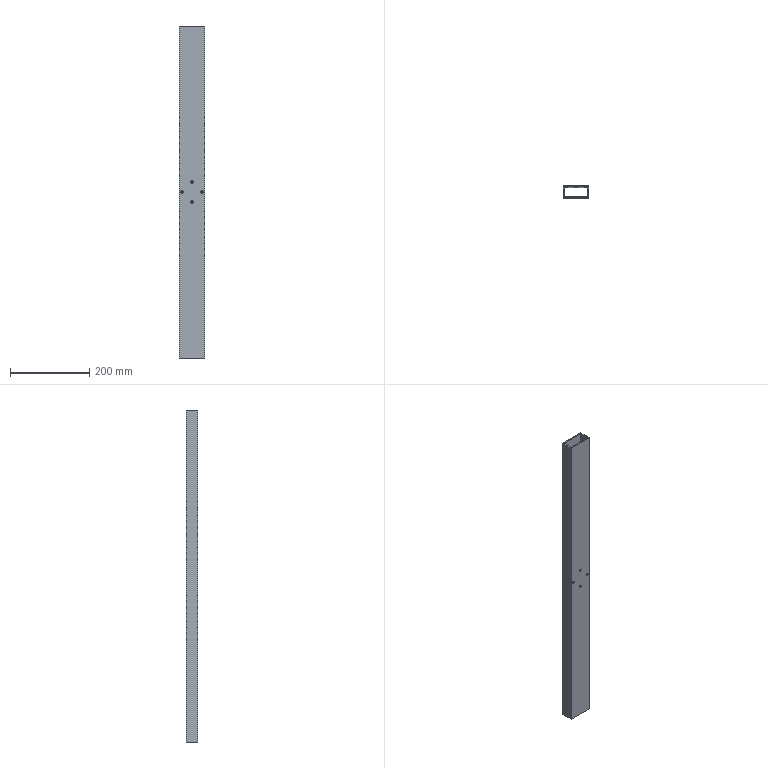Part | SolidWorks | features ICE 2, Extrusion 1 | 1 solid | 26 faces | box 65 x 30 x 840 mm | volume 447881 mm3 | cylinder 16 | plane 10 | commonest cylinder face diameters 6 x16
STEP:
#1=CARTESIAN_POINT('',(-8.041,12.808,398.));
#2=VERTEX_POINT('',#1);
#3=CARTESIAN_POINT('',(-8.041,12.808,392.));
#4=VERTEX_POINT('',#3);
#5=CARTESIAN_POINT('',(-8.041,12.808,395.));
#6=DIRECTION('',(0.,-1.,0.));
#7=DIRECTION('',(1.,0.,0.));
#8=AXIS2_PLACEMENT_3D('',#5,#6,#7);
#9=CIRCLE('',#8,3.);
#10=EDGE_CURVE('',#2,#4,#9,.T.);
#11=ORIENTED_EDGE('',*,*,#10,.F.);
#12=CARTESIAN_POINT('',(-8.041,9.808,398.));
#13=VERTEX_POINT('',#12);
#14=CARTESIAN_POINT('',(-8.041,39.808,398.));
#15=DIRECTION('',(0.,-1.,0.));
#16=VECTOR('',#15,1000.);
#17=LINE('',#14,#16);
#18=EDGE_CURVE('',#2,#13,#17,.T.);
#19=ORIENTED_EDGE('',*,*,#18,.T.);
#20=CARTESIAN_POINT('',(-8.041,9.808,392.));
#21=VERTEX_POINT('',#20);
#22=CARTESIAN_POINT('',(-8.041,9.808,395.));
#23=DIRECTION('',(0.,-1.,0.));
#24=DIRECTION('',(0.,0.,-1.));
#25=AXIS2_PLACEMENT_3D('',#22,#23,#24);
#26=CIRCLE('',#25,3.);
#27=EDGE_CURVE('',#13,#21,#26,.T.);
#28=ORIENTED_EDGE('',*,*,#27,.T.);
#29=CARTESIAN_POINT('',(-8.041,39.808,392.));
#30=DIRECTION('',(0.,-1.,0.));
#31=VECTOR('',#30,1000.);
#32=LINE('',#29,#31);
#33=EDGE_CURVE('',#4,#21,#32,.T.);
#34=ORIENTED_EDGE('',*,*,#33,.F.);
#35=EDGE_LOOP('',(#11,#19,#28,#34));
#36=FACE_OUTER_BOUND('',#35,.T.);
#37=CARTESIAN_POINT('',(-8.041,39.808,395.));
#38=DIRECTION('',(0.,-1.,0.));
#39=DIRECTION('',(0.,0.,-1.));
#40=AXIS2_PLACEMENT_3D('',#37,#38,#39);
#41=CYLINDRICAL_SURFACE('',#40,3.);
#42=ADVANCED_FACE('',(#36),#41,.F.);
#43=CARTESIAN_POINT('',(-33.041,12.808,423.));
#44=VERTEX_POINT('',#43);
#45=CARTESIAN_POINT('',(-33.041,12.808,417.));
#46=VERTEX_POINT('',#45);
#47=CARTESIAN_POINT('',(-33.041,12.808,420.));
#48=DIRECTION('',(0.,-1.,0.));
#49=DIRECTION('',(1.,0.,0.));
#50=AXIS2_PLACEMENT_3D('',#47,#48,#49);
#51=CIRCLE('',#50,3.);
#52=EDGE_CURVE('',#44,#46,#51,.T.);
#53=ORIENTED_EDGE('',*,*,#52,.F.);
#54=CARTESIAN_POINT('',(-33.041,9.808,423.));
#55=VERTEX_POINT('',#54);
#56=CARTESIAN_POINT('',(-33.041,39.808,423.));
#57=DIRECTION('',(0.,-1.,0.));
#58=VECTOR('',#57,1000.);
#59=LINE('',#56,#58);
#60=EDGE_CURVE('',#44,#55,#59,.T.);
#61=ORIENTED_EDGE('',*,*,#60,.T.);
#62=CARTESIAN_POINT('',(-33.041,9.808,417.));
#63=VERTEX_POINT('',#62);
#64=CARTESIAN_POINT('',(-33.041,9.808,420.));
#65=DIRECTION('',(0.,-1.,0.));
#66=DIRECTION('',(0.,0.,-1.));
#67=AXIS2_PLACEMENT_3D('',#64,#65,#66);
#68=CIRCLE('',#67,3.);
#69=EDGE_CURVE('',#55,#63,#68,.T.);
#70=ORIENTED_EDGE('',*,*,#69,.T.);
#71=CARTESIAN_POINT('',(-33.041,39.808,417.));
#72=DIRECTION('',(0.,-1.,0.));
#73=VECTOR('',#72,1000.);
#74=LINE('',#71,#73);
#75=EDGE_CURVE('',#46,#63,#74,.T.);
#76=ORIENTED_EDGE('',*,*,#75,.F.);
#77=EDGE_LOOP('',(#53,#61,#70,#76));
#78=FACE_OUTER_BOUND('',#77,.T.);
#79=CARTESIAN_POINT('',(-33.041,39.808,420.));
#80=DIRECTION('',(0.,-1.,0.));
#81=DIRECTION('',(0.,0.,-1.));
#82=AXIS2_PLACEMENT_3D('',#79,#80,#81);
#83=CYLINDRICAL_SURFACE('',#82,3.);
#84=ADVANCED_FACE('',(#78),#83,.F.);
#85=CARTESIAN_POINT('',(-8.041,12.808,448.));
#86=VERTEX_POINT('',#85);
#87=CARTESIAN_POINT('',(-8.041,12.808,442.));
#88=VERTEX_POINT('',#87);
#89=CARTESIAN_POINT('',(-8.041,12.808,445.));
#90=DIRECTION('',(0.,-1.,0.));
#91=DIRECTION('',(1.,0.,0.));
#92=AXIS2_PLACEMENT_3D('',#89,#90,#91);
#93=CIRCLE('',#92,3.);
#94=EDGE_CURVE('',#86,#88,#93,.T.);
#95=ORIENTED_EDGE('',*,*,#94,.F.);
#96=CARTESIAN_POINT('',(-8.041,9.808,448.));
#97=VERTEX_POINT('',#96);
#98=CARTESIAN_POINT('',(-8.041,39.808,448.));
#99=DIRECTION('',(0.,-1.,0.));
#100=VECTOR('',#99,1000.);
#101=LINE('',#98,#100);
#102=EDGE_CURVE('',#86,#97,#101,.T.);
#103=ORIENTED_EDGE('',*,*,#102,.T.);
#104=CARTESIAN_POINT('',(-8.041,9.808,442.));
#105=VERTEX_POINT('',#104);
#106=CARTESIAN_POINT('',(-8.041,9.808,445.));
#107=DIRECTION('',(0.,-1.,0.));
#108=DIRECTION('',(0.,0.,-1.));
#109=AXIS2_PLACEMENT_3D('',#106,#107,#108);
#110=CIRCLE('',#109,3.);
#111=EDGE_CURVE('',#97,#105,#110,.T.);
#112=ORIENTED_EDGE('',*,*,#111,.T.);
#113=CARTESIAN_POINT('',(-8.041,39.808,442.));
#114=DIRECTION('',(0.,-1.,0.));
#115=VECTOR('',#114,1000.);
#116=LINE('',#113,#115);
#117=EDGE_CURVE('',#88,#105,#116,.T.);
#118=ORIENTED_EDGE('',*,*,#117,.F.);
#119=EDGE_LOOP('',(#95,#103,#112,#118));
#120=FACE_OUTER_BOUND('',#119,.T.);
#121=CARTESIAN_POINT('',(-8.041,39.808,445.));
#122=DIRECTION('',(0.,-1.,0.));
#123=DIRECTION('',(0.,0.,-1.));
#124=AXIS2_PLACEMENT_3D('',#121,#122,#123);
#125=CYLINDRICAL_SURFACE('',#124,3.);
#126=ADVANCED_FACE('',(#120),#125,.F.);
#127=CARTESIAN_POINT('',(16.959,12.808,423.));
#128=VERTEX_POINT('',#127);
#129=CARTESIAN_POINT('',(16.959,12.808,417.));
#130=VERTEX_POINT('',#129);
#131=CARTESIAN_POINT('',(16.959,12.808,420.));
#132=DIRECTION('',(0.,-1.,0.));
#133=DIRECTION('',(1.,0.,0.));
#134=AXIS2_PLACEMENT_3D('',#131,#132,#133);
#135=CIRCLE('',#134,3.);
#136=EDGE_CURVE('',#128,#130,#135,.T.);
#137=ORIENTED_EDGE('',*,*,#136,.F.);
#138=CARTESIAN_POINT('',(16.959,9.808,423.));
#139=VERTEX_POINT('',#138);
#140=CARTESIAN_POINT('',(16.959,39.808,423.));
#141=DIRECTION('',(0.,-1.,0.));
#142=VECTOR('',#141,1000.);
#143=LINE('',#140,#142);
#144=EDGE_CURVE('',#128,#139,#143,.T.);
#145=ORIENTED_EDGE('',*,*,#144,.T.);
#146=CARTESIAN_POINT('',(16.959,9.808,417.));
#147=VERTEX_POINT('',#146);
#148=CARTESIAN_POINT('',(16.959,9.808,420.));
#149=DIRECTION('',(0.,-1.,0.));
#150=DIRECTION('',(0.,0.,-1.));
#151=AXIS2_PLACEMENT_3D('',#148,#149,#150);
#152=CIRCLE('',#151,3.);
#153=EDGE_CURVE('',#139,#147,#152,.T.);
#154=ORIENTED_EDGE('',*,*,#153,.T.);
#155=CARTESIAN_POINT('',(16.959,39.808,417.));
#156=DIRECTION('',(0.,-1.,0.));
#157=VECTOR('',#156,1000.);
#158=LINE('',#155,#157);
#159=EDGE_CURVE('',#130,#147,#158,.T.);
#160=ORIENTED_EDGE('',*,*,#159,.F.);
#161=EDGE_LOOP('',(#137,#145,#154,#160));
#162=FACE_OUTER_BOUND('',#161,.T.);
#163=CARTESIAN_POINT('',(16.959,39.808,420.));
#164=DIRECTION('',(0.,-1.,0.));
#165=DIRECTION('',(0.,0.,-1.));
#166=AXIS2_PLACEMENT_3D('',#163,#164,#165);
#167=CYLINDRICAL_SURFACE('',#166,3.);
#168=ADVANCED_FACE('',(#162),#167,.F.);
#169=CARTESIAN_POINT('',(-8.041,39.808,398.));
#170=VERTEX_POINT('',#169);
#171=CARTESIAN_POINT('',(-8.041,39.808,392.));
#172=VERTEX_POINT('',#171);
#173=CARTESIAN_POINT('',(-8.041,39.808,395.));
#174=DIRECTION('',(0.,-1.,0.));
#175=DIRECTION('',(0.,0.,-1.));
#176=AXIS2_PLACEMENT_3D('',#173,#174,#175);
#177=CIRCLE('',#176,3.);
#178=EDGE_CURVE('',#170,#172,#177,.T.);
#179=ORIENTED_EDGE('',*,*,#178,.F.);
#180=CARTESIAN_POINT('',(-8.041,36.808,398.));
#181=VERTEX_POINT('',#180);
#182=CARTESIAN_POINT('',(-8.041,39.808,398.));
#183=DIRECTION('',(0.,-1.,0.));
#184=VECTOR('',#183,1000.);
#185=LINE('',#182,#184);
#186=EDGE_CURVE('',#170,#181,#185,.T.);
#187=ORIENTED_EDGE('',*,*,#186,.T.);
#188=CARTESIAN_POINT('',(-8.041,36.808,392.));
#189=VERTEX_POINT('',#188);
#190=CARTESIAN_POINT('',(-8.041,36.808,395.));
#191=DIRECTION('',(0.,1.,0.));
#192=DIRECTION('',(-1.,0.,0.));
#193=AXIS2_PLACEMENT_3D('',#190,#191,#192);
#194=CIRCLE('',#193,3.);
#195=EDGE_CURVE('',#189,#181,#194,.T.);
#196=ORIENTED_EDGE('',*,*,#195,.F.);
#197=CARTESIAN_POINT('',(-8.041,39.808,392.));
#198=DIRECTION('',(0.,-1.,0.));
#199=VECTOR('',#198,1000.);
#200=LINE('',#197,#199);
#201=EDGE_CURVE('',#172,#189,#200,.T.);
#202=ORIENTED_EDGE('',*,*,#201,.F.);
#203=EDGE_LOOP('',(#179,#187,#196,#202));
#204=FACE_OUTER_BOUND('',#203,.T.);
#205=CARTESIAN_POINT('',(-8.041,39.808,395.));
#206=DIRECTION('',(0.,-1.,0.));
#207=DIRECTION('',(0.,0.,-1.));
#208=AXIS2_PLACEMENT_3D('',#205,#206,#207);
#209=CYLINDRICAL_SURFACE('',#208,3.);
#210=ADVANCED_FACE('',(#204),#209,.F.);
#211=CARTESIAN_POINT('',(-33.041,39.808,423.));
#212=VERTEX_POINT('',#211);
#213=CARTESIAN_POINT('',(-33.041,39.808,417.));
#214=VERTEX_POINT('',#213);
#215=CARTESIAN_POINT('',(-33.041,39.808,420.));
#216=DIRECTION('',(0.,-1.,0.));
#217=DIRECTION('',(0.,0.,-1.));
#218=AXIS2_PLACEMENT_3D('',#215,#216,#217);
#219=CIRCLE('',#218,3.);
#220=EDGE_CURVE('',#212,#214,#219,.T.);
#221=ORIENTED_EDGE('',*,*,#220,.F.);
#222=CARTESIAN_POINT('',(-33.041,36.808,423.));
#223=VERTEX_POINT('',#222);
#224=CARTESIAN_POINT('',(-33.041,39.808,423.));
#225=DIRECTION('',(0.,-1.,0.));
#226=VECTOR('',#225,1000.);
#227=LINE('',#224,#226);
#228=EDGE_CURVE('',#212,#223,#227,.T.);
#229=ORIENTED_EDGE('',*,*,#228,.T.);
#230=CARTESIAN_POINT('',(-33.041,36.808,417.));
#231=VERTEX_POINT('',#230);
#232=CARTESIAN_POINT('',(-33.041,36.808,420.));
#233=DIRECTION('',(0.,1.,0.));
#234=DIRECTION('',(-1.,0.,0.));
#235=AXIS2_PLACEMENT_3D('',#232,#233,#234);
#236=CIRCLE('',#235,3.);
#237=EDGE_CURVE('',#231,#223,#236,.T.);
#238=ORIENTED_EDGE('',*,*,#237,.F.);
#239=CARTESIAN_POINT('',(-33.041,39.808,417.));
#240=DIRECTION('',(0.,-1.,0.));
#241=VECTOR('',#240,1000.);
#242=LINE('',#239,#241);
#243=EDGE_CURVE('',#214,#231,#242,.T.);
#244=ORIENTED_EDGE('',*,*,#243,.F.);
#245=EDGE_LOOP('',(#221,#229,#238,#244));
#246=FACE_OUTER_BOUND('',#245,.T.);
#247=CARTESIAN_POINT('',(-33.041,39.808,420.));
#248=DIRECTION('',(0.,-1.,0.));
#249=DIRECTION('',(0.,0.,-1.));
#250=AXIS2_PLACEMENT_3D('',#247,#248,#249);
#251=CYLINDRICAL_SURFACE('',#250,3.);
#252=ADVANCED_FACE('',(#246),#251,.F.);
#253=CARTESIAN_POINT('',(-8.041,39.808,448.));
#254=VERTEX_POINT('',#253);
#255=CARTESIAN_POINT('',(-8.041,39.808,442.));
#256=VERTEX_POINT('',#255);
#257=CARTESIAN_POINT('',(-8.041,39.808,445.));
#258=DIRECTION('',(0.,-1.,0.));
#259=DIRECTION('',(0.,0.,-1.));
#260=AXIS2_PLACEMENT_3D('',#257,#258,#259);
#261=CIRCLE('',#260,3.);
#262=EDGE_CURVE('',#254,#256,#261,.T.);
#263=ORIENTED_EDGE('',*,*,#262,.F.);
#264=CARTESIAN_POINT('',(-8.041,36.808,448.));
#265=VERTEX_POINT('',#264);
#266=CARTESIAN_POINT('',(-8.041,39.808,448.));
#267=DIRECTION('',(0.,-1.,0.));
#268=VECTOR('',#267,1000.);
#269=LINE('',#266,#268);
#270=EDGE_CURVE('',#254,#265,#269,.T.);
#271=ORIENTED_EDGE('',*,*,#270,.T.);
#272=CARTESIAN_POINT('',(-8.041,36.808,442.));
#273=VERTEX_POINT('',#272);
#274=CARTESIAN_POINT('',(-8.041,36.808,445.));
#275=DIRECTION('',(0.,1.,0.));
#276=DIRECTION('',(-1.,0.,0.));
#277=AXIS2_PLACEMENT_3D('',#274,#275,#276);
#278=CIRCLE('',#277,3.);
#279=EDGE_CURVE('',#273,#265,#278,.T.);
#280=ORIENTED_EDGE('',*,*,#279,.F.);
#281=CARTESIAN_POINT('',(-8.041,39.808,442.));
#282=DIRECTION('',(0.,-1.,0.));
#283=VECTOR('',#282,1000.);
#284=LINE('',#281,#283);
#285=EDGE_CURVE('',#256,#273,#284,.T.);
#286=ORIENTED_EDGE('',*,*,#285,.F.);
#287=EDGE_LOOP('',(#263,#271,#280,#286));
#288=FACE_OUTER_BOUND('',#287,.T.);
#289=CARTESIAN_POINT('',(-8.041,39.808,445.));
#290=DIRECTION('',(0.,-1.,0.));
#291=DIRECTION('',(0.,0.,-1.));
#292=AXIS2_PLACEMENT_3D('',#289,#290,#291);
#293=CYLINDRICAL_SURFACE('',#292,3.);
#294=ADVANCED_FACE('',(#288),#293,.F.);
#295=CARTESIAN_POINT('',(16.959,39.808,423.));
#296=VERTEX_POINT('',#295);
#297=CARTESIAN_POINT('',(16.959,39.808,417.));
#298=VERTEX_POINT('',#297);
#299=CARTESIAN_POINT('',(16.959,39.808,420.));
#300=DIRECTION('',(0.,-1.,0.));
#301=DIRECTION('',(0.,0.,-1.));
#302=AXIS2_PLACEMENT_3D('',#299,#300,#301);
#303=CIRCLE('',#302,3.);
#304=EDGE_CURVE('',#296,#298,#303,.T.);
#305=ORIENTED_EDGE('',*,*,#304,.F.);
#306=CARTESIAN_POINT('',(16.959,36.808,423.));
#307=VERTEX_POINT('',#306);
#308=CARTESIAN_POINT('',(16.959,39.808,423.));
#309=DIRECTION('',(0.,-1.,0.));
#310=VECTOR('',#309,1000.);
#311=LINE('',#308,#310);
#312=EDGE_CURVE('',#296,#307,#311,.T.);
#313=ORIENTED_EDGE('',*,*,#312,.T.);
#314=CARTESIAN_POINT('',(16.959,36.808,417.));
#315=VERTEX_POINT('',#314);
#316=CARTESIAN_POINT('',(16.959,36.808,420.));
#317=DIRECTION('',(0.,1.,0.));
#318=DIRECTION('',(-1.,0.,0.));
#319=AXIS2_PLACEMENT_3D('',#316,#317,#318);
#320=CIRCLE('',#319,3.);
#321=EDGE_CURVE('',#315,#307,#320,.T.);
#322=ORIENTED_EDGE('',*,*,#321,.F.);
#323=CARTESIAN_POINT('',(16.959,39.808,417.));
#324=DIRECTION('',(0.,-1.,0.));
#325=VECTOR('',#324,1000.);
#326=LINE('',#323,#325);
#327=EDGE_CURVE('',#298,#315,#326,.T.);
#328=ORIENTED_EDGE('',*,*,#327,.F.);
#329=EDGE_LOOP('',(#305,#313,#322,#328));
#330=FACE_OUTER_BOUND('',#329,.T.);
#331=CARTESIAN_POINT('',(16.959,39.808,420.));
#332=DIRECTION('',(0.,-1.,0.));
#333=DIRECTION('',(0.,0.,-1.));
#334=AXIS2_PLACEMENT_3D('',#331,#332,#333);
#335=CYLINDRICAL_SURFACE('',#334,3.);
#336=ADVANCED_FACE('',(#330),#335,.F.);
#337=CARTESIAN_POINT('',(-40.541,39.808,0.));
#338=VERTEX_POINT('',#337);
#339=CARTESIAN_POINT('',(-40.541,9.808,0.));
#340=VERTEX_POINT('',#339);
#341=CARTESIAN_POINT('',(-40.541,9.808,0.));
#342=DIRECTION('',(0.,-1.,0.));
#343=VECTOR('',#342,1000.);
#344=LINE('',#341,#343);
#345=EDGE_CURVE('',#338,#340,#344,.T.);
#346=ORIENTED_EDGE('',*,*,#345,.T.);
#347=CARTESIAN_POINT('',(-40.541,9.808,840.));
#348=VERTEX_POINT('',#347);
#349=CARTESIAN_POINT('',(-40.541,9.808,840.));
#350=DIRECTION('',(0.,0.,-1.));
#351=VECTOR('',#350,1000.);
#352=LINE('',#349,#351);
#353=EDGE_CURVE('',#348,#340,#352,.T.);
#354=ORIENTED_EDGE('',*,*,#353,.F.);
#355=CARTESIAN_POINT('',(-40.541,39.808,840.));
#356=VERTEX_POINT('',#355);
#357=CARTESIAN_POINT('',(-40.541,9.808,840.));
#358=DIRECTION('',(0.,-1.,0.));
#359=VECTOR('',#358,1000.);
#360=LINE('',#357,#359);
#361=EDGE_CURVE('',#356,#348,#360,.T.);
#362=ORIENTED_EDGE('',*,*,#361,.F.);
#363=CARTESIAN_POINT('',(-40.541,39.808,840.));
#364=DIRECTION('',(0.,0.,-1.));
#365=VECTOR('',#364,1000.);
#366=LINE('',#363,#365);
#367=EDGE_CURVE('',#356,#338,#366,.T.);
#368=ORIENTED_EDGE('',*,*,#367,.T.);
#369=EDGE_LOOP('',(#346,#354,#362,#368));
#370=FACE_OUTER_BOUND('',#369,.T.);
#371=CARTESIAN_POINT('',(-40.541,9.808,840.));
#372=DIRECTION('',(1.,0.,0.));
#373=DIRECTION('',(0.,0.,-1.));
#374=AXIS2_PLACEMENT_3D('',#371,#372,#373);
#375=PLANE('',#374);
#376=ADVANCED_FACE('',(#370),#375,.F.);
#377=CARTESIAN_POINT('',(-8.041,9.808,395.));
#378=DIRECTION('',(0.,-1.,0.));
#379=DIRECTION('',(0.,0.,-1.));
#380=AXIS2_PLACEMENT_3D('',#377,#378,#379);
#381=CIRCLE('',#380,3.);
#382=EDGE_CURVE('',#21,#13,#381,.T.);
#383=ORIENTED_EDGE('',*,*,#382,.F.);
#384=ORIENTED_EDGE('',*,*,#27,.F.);
#385=EDGE_LOOP('',(#383,#384));
#386=FACE_BOUND('',#385,.T.);
#387=CARTESIAN_POINT('',(-33.041,9.808,420.));
#388=DIRECTION('',(0.,-1.,0.));
#389=DIRECTION('',(0.,0.,-1.));
#390=AXIS2_PLACEMENT_3D('',#387,#388,#389);
#391=CIRCLE('',#390,3.);
#392=EDGE_CURVE('',#63,#55,#391,.T.);
#393=ORIENTED_EDGE('',*,*,#392,.F.);
#394=ORIENTED_EDGE('',*,*,#69,.F.);
#395=EDGE_LOOP('',(#393,#394));
#396=FACE_BOUND('',#395,.T.);
#397=CARTESIAN_POINT('',(-8.041,9.808,445.));
#398=DIRECTION('',(0.,-1.,0.));
#399=DIRECTION('',(0.,0.,-1.));
#400=AXIS2_PLACEMENT_3D('',#397,#398,#399);
#401=CIRCLE('',#400,3.);
#402=EDGE_CURVE('',#105,#97,#401,.T.);
#403=ORIENTED_EDGE('',*,*,#402,.F.);
#404=ORIENTED_EDGE('',*,*,#111,.F.);
#405=EDGE_LOOP('',(#403,#404));
#406=FACE_BOUND('',#405,.T.);
#407=CARTESIAN_POINT('',(16.959,9.808,420.));
#408=DIRECTION('',(0.,-1.,0.));
#409=DIRECTION('',(0.,0.,-1.));
#410=AXIS2_PLACEMENT_3D('',#407,#408,#409);
#411=CIRCLE('',#410,3.);
#412=EDGE_CURVE('',#147,#139,#411,.T.);
#413=ORIENTED_EDGE('',*,*,#412,.F.);
#414=ORIENTED_EDGE('',*,*,#153,.F.);
#415=EDGE_LOOP('',(#413,#414));
#416=FACE_BOUND('',#415,.T.);
#417=CARTESIAN_POINT('',(24.459,9.808,0.));
#418=VERTEX_POINT('',#417);
#419=CARTESIAN_POINT('',(24.459,9.808,0.));
#420=DIRECTION('',(1.,0.,0.));
#421=VECTOR('',#420,1000.);
#422=LINE('',#419,#421);
#423=EDGE_CURVE('',#340,#418,#422,.T.);
#424=ORIENTED_EDGE('',*,*,#423,.T.);
#425=CARTESIAN_POINT('',(24.459,9.808,840.));
#426=VERTEX_POINT('',#425);
#427=CARTESIAN_POINT('',(24.459,9.808,840.));
#428=DIRECTION('',(0.,0.,-1.));
#429=VECTOR('',#428,1000.);
#430=LINE('',#427,#429);
#431=EDGE_CURVE('',#426,#418,#430,.T.);
#432=ORIENTED_EDGE('',*,*,#431,.F.);
#433=CARTESIAN_POINT('',(24.459,9.808,840.));
#434=DIRECTION('',(1.,0.,0.));
#435=VECTOR('',#434,1000.);
#436=LINE('',#433,#435);
#437=EDGE_CURVE('',#348,#426,#436,.T.);
#438=ORIENTED_EDGE('',*,*,#437,.F.);
#439=ORIENTED_EDGE('',*,*,#353,.T.);
#440=EDGE_LOOP('',(#424,#432,#438,#439));
#441=FACE_OUTER_BOUND('',#440,.T.);
#442=CARTESIAN_POINT('',(24.459,9.808,840.));
#443=DIRECTION('',(0.,1.,0.));
#444=DIRECTION('',(0.,0.,1.));
#445=AXIS2_PLACEMENT_3D('',#442,#443,#444);
#446=PLANE('',#445);
#447=ADVANCED_FACE('',(#386,#396,#406,#416,#441),#446,.F.);
#448=CARTESIAN_POINT('',(24.459,39.808,0.));
#449=VERTEX_POINT('',#448);
#450=CARTESIAN_POINT('',(24.459,39.808,0.));
#451=DIRECTION('',(0.,1.,0.));
#452=VECTOR('',#451,1000.);
#453=LINE('',#450,#452);
#454=EDGE_CURVE('',#418,#449,#453,.T.);
#455=ORIENTED_EDGE('',*,*,#454,.T.);
#456=CARTESIAN_POINT('',(24.459,39.808,840.));
#457=VERTEX_POINT('',#456);
#458=CARTESIAN_POINT('',(24.459,39.808,840.));
#459=DIRECTION('',(0.,0.,-1.));
#460=VECTOR('',#459,1000.);
#461=LINE('',#458,#460);
#462=EDGE_CURVE('',#457,#449,#461,.T.);
#463=ORIENTED_EDGE('',*,*,#462,.F.);
#464=CARTESIAN_POINT('',(24.459,39.808,840.));
#465=DIRECTION('',(0.,1.,0.));
#466=VECTOR('',#465,1000.);
#467=LINE('',#464,#466);
#468=EDGE_CURVE('',#426,#457,#467,.T.);
#469=ORIENTED_EDGE('',*,*,#468,.F.);
#470=ORIENTED_EDGE('',*,*,#431,.T.);
#471=EDGE_LOOP('',(#455,#463,#469,#470));
#472=FACE_OUTER_BOUND('',#471,.T.);
#473=CARTESIAN_POINT('',(24.459,39.808,840.));
#474=DIRECTION('',(-1.,0.,0.));
#475=DIRECTION('',(0.,0.,1.));
#476=AXIS2_PLACEMENT_3D('',#473,#474,#475);
#477=PLANE('',#476);
#478=ADVANCED_FACE('',(#472),#477,.F.);
#479=CARTESIAN_POINT('',(-8.041,39.808,395.));
#480=DIRECTION('',(0.,-1.,0.));
#481=DIRECTION('',(0.,0.,-1.));
#482=AXIS2_PLACEMENT_3D('',#479,#480,#481);
#483=CIRCLE('',#482,3.);
#484=EDGE_CURVE('',#172,#170,#483,.T.);
#485=ORIENTED_EDGE('',*,*,#484,.T.);
#486=ORIENTED_EDGE('',*,*,#178,.T.);
#487=EDGE_LOOP('',(#485,#486));
#488=FACE_BOUND('',#487,.T.);
#489=CARTESIAN_POINT('',(-33.041,39.808,420.));
#490=DIRECTION('',(0.,-1.,0.));
#491=DIRECTION('',(0.,0.,-1.));
#492=AXIS2_PLACEMENT_3D('',#489,#490,#491);
#493=CIRCLE('',#492,3.);
#494=EDGE_CURVE('',#214,#212,#493,.T.);
#495=ORIENTED_EDGE('',*,*,#494,.T.);
#496=ORIENTED_EDGE('',*,*,#220,.T.);
#497=EDGE_LOOP('',(#495,#496));
#498=FACE_BOUND('',#497,.T.);
#499=CARTESIAN_POINT('',(-8.041,39.808,445.));
#500=DIRECTION('',(0.,-1.,0.));
#501=DIRECTION('',(0.,0.,-1.));
#502=AXIS2_PLACEMENT_3D('',#499,#500,#501);
#503=CIRCLE('',#502,3.);
#504=EDGE_CURVE('',#256,#254,#503,.T.);
#505=ORIENTED_EDGE('',*,*,#504,.T.);
#506=ORIENTED_EDGE('',*,*,#262,.T.);
#507=EDGE_LOOP('',(#505,#506));
#508=FACE_BOUND('',#507,.T.);
#509=CARTESIAN_POINT('',(16.959,39.808,420.));
#510=DIRECTION('',(0.,-1.,0.));
#511=DIRECTION('',(0.,0.,-1.));
#512=AXIS2_PLACEMENT_3D('',#509,#510,#511);
#513=CIRCLE('',#512,3.);
#514=EDGE_CURVE('',#298,#296,#513,.T.);
#515=ORIENTED_EDGE('',*,*,#514,.T.);
#516=ORIENTED_EDGE('',*,*,#304,.T.);
#517=EDGE_LOOP('',(#515,#516));
#518=FACE_BOUND('',#517,.T.);
#519=CARTESIAN_POINT('',(-40.541,39.808,0.));
#520=DIRECTION('',(-1.,0.,0.));
#521=VECTOR('',#520,1000.);
#522=LINE('',#519,#521);
#523=EDGE_CURVE('',#449,#338,#522,.T.);
#524=ORIENTED_EDGE('',*,*,#523,.T.);
#525=ORIENTED_EDGE('',*,*,#367,.F.);
#526=CARTESIAN_POINT('',(-40.541,39.808,840.));
#527=DIRECTION('',(-1.,0.,0.));
#528=VECTOR('',#527,1000.);
#529=LINE('',#526,#528);
#530=EDGE_CURVE('',#457,#356,#529,.T.);
#531=ORIENTED_EDGE('',*,*,#530,.F.);
#532=ORIENTED_EDGE('',*,*,#462,.T.);
#533=EDGE_LOOP('',(#524,#525,#531,#532));
#534=FACE_OUTER_BOUND('',#533,.T.);
#535=CARTESIAN_POINT('',(-40.541,39.808,840.));
#536=DIRECTION('',(0.,-1.,0.));
#537=DIRECTION('',(0.,0.,-1.));
#538=AXIS2_PLACEMENT_3D('',#535,#536,#537);
#539=PLANE('',#538);
#540=ADVANCED_FACE('',(#488,#498,#508,#518,#534),#539,.F.);
#541=CARTESIAN_POINT('',(21.459,36.808,840.));
#542=VERTEX_POINT('',#541);
#543=CARTESIAN_POINT('',(-37.541,36.808,840.));
#544=VERTEX_POINT('',#543);
#545=CARTESIAN_POINT('',(-37.541,36.808,840.));
#546=DIRECTION('',(-1.,0.,0.));
#547=VECTOR('',#546,1000.);
#548=LINE('',#545,#547);
#549=EDGE_CURVE('',#542,#544,#548,.T.);
#550=ORIENTED_EDGE('',*,*,#549,.F.);
#551=CARTESIAN_POINT('',(21.459,12.808,840.));
#552=VERTEX_POINT('',#551);
#553=CARTESIAN_POINT('',(21.459,36.808,840.));
#554=DIRECTION('',(0.,1.,0.));
#555=VECTOR('',#554,1000.);
#556=LINE('',#553,#555);
#557=EDGE_CURVE('',#552,#542,#556,.T.);
#558=ORIENTED_EDGE('',*,*,#557,.F.);
#559=CARTESIAN_POINT('',(-37.541,12.808,840.));
#560=VERTEX_POINT('',#559);
#561=CARTESIAN_POINT('',(21.459,12.808,840.));
#562=DIRECTION('',(1.,0.,0.));
#563=VECTOR('',#562,1000.);
#564=LINE('',#561,#563);
#565=EDGE_CURVE('',#560,#552,#564,.T.);
#566=ORIENTED_EDGE('',*,*,#565,.F.);
#567=CARTESIAN_POINT('',(-37.541,12.808,840.));
#568=DIRECTION('',(0.,-1.,0.));
#569=VECTOR('',#568,1000.);
#570=LINE('',#567,#569);
#571=EDGE_CURVE('',#544,#560,#570,.T.);
#572=ORIENTED_EDGE('',*,*,#571,.F.);
#573=EDGE_LOOP('',(#550,#558,#566,#572));
#574=FACE_BOUND('',#573,.T.);
#575=ORIENTED_EDGE('',*,*,#361,.T.);
#576=ORIENTED_EDGE('',*,*,#437,.T.);
#577=ORIENTED_EDGE('',*,*,#468,.T.);
#578=ORIENTED_EDGE('',*,*,#530,.T.);
#579=EDGE_LOOP('',(#575,#576,#577,#578));
#580=FACE_OUTER_BOUND('',#579,.T.);
#581=CARTESIAN_POINT('',(0.,0.,840.));
#582=DIRECTION('',(0.,0.,-1.));
#583=DIRECTION('',(-1.,0.,0.));
#584=AXIS2_PLACEMENT_3D('',#581,#582,#583);
#585=PLANE('',#584);
#586=ADVANCED_FACE('',(#574,#580),#585,.F.);
#587=CARTESIAN_POINT('',(21.459,36.808,0.));
#588=VERTEX_POINT('',#587);
#589=CARTESIAN_POINT('',(21.459,12.808,0.));
#590=VERTEX_POINT('',#589);
#591=CARTESIAN_POINT('',(21.459,0.,0.));
#592=DIRECTION('',(0.,-1.,0.));
#593=VECTOR('',#592,1000.);
#594=LINE('',#591,#593);
#595=EDGE_CURVE('',#588,#590,#594,.T.);
#596=ORIENTED_EDGE('',*,*,#595,.F.);
#597=CARTESIAN_POINT('',(-37.541,36.808,0.));
#598=VERTEX_POINT('',#597);
#599=CARTESIAN_POINT('',(0.,36.808,0.));
#600=DIRECTION('',(1.,0.,0.));
#601=VECTOR('',#600,1000.);
#602=LINE('',#599,#601);
#603=EDGE_CURVE('',#598,#588,#602,.T.);
#604=ORIENTED_EDGE('',*,*,#603,.F.);
#605=CARTESIAN_POINT('',(-37.541,12.808,0.));
#606=VERTEX_POINT('',#605);
#607=CARTESIAN_POINT('',(-37.541,0.,0.));
#608=DIRECTION('',(0.,1.,0.));
#609=VECTOR('',#608,1000.);
#610=LINE('',#607,#609);
#611=EDGE_CURVE('',#606,#598,#610,.T.);
#612=ORIENTED_EDGE('',*,*,#611,.F.);
#613=CARTESIAN_POINT('',(0.,12.808,0.));
#614=DIRECTION('',(-1.,0.,0.));
#615=VECTOR('',#614,1000.);
#616=LINE('',#613,#615);
#617=EDGE_CURVE('',#590,#606,#616,.T.);
#618=ORIENTED_EDGE('',*,*,#617,.F.);
#619=EDGE_LOOP('',(#596,#604,#612,#618));
#620=FACE_BOUND('',#619,.T.);
#621=ORIENTED_EDGE('',*,*,#345,.F.);
#622=ORIENTED_EDGE('',*,*,#523,.F.);
#623=ORIENTED_EDGE('',*,*,#454,.F.);
#624=ORIENTED_EDGE('',*,*,#423,.F.);
#625=EDGE_LOOP('',(#621,#622,#623,#624));
#626=FACE_OUTER_BOUND('',#625,.T.);
#627=CARTESIAN_POINT('',(0.,0.,0.));
#628=DIRECTION('',(0.,0.,-1.));
#629=DIRECTION('',(-1.,0.,0.));
#630=AXIS2_PLACEMENT_3D('',#627,#628,#629);
#631=PLANE('',#630);
#632=ADVANCED_FACE('',(#620,#626),#631,.T.);
#633=ORIENTED_EDGE('',*,*,#595,.T.);
#634=CARTESIAN_POINT('',(21.459,12.808,-110.));
#635=DIRECTION('',(0.,0.,1.));
#636=VECTOR('',#635,1000.);
#637=LINE('',#634,#636);
#638=EDGE_CURVE('',#590,#552,#637,.T.);
#639=ORIENTED_EDGE('',*,*,#638,.T.);
#640=ORIENTED_EDGE('',*,*,#557,.T.);
#641=CARTESIAN_POINT('',(21.459,36.808,-110.));
#642=DIRECTION('',(0.,0.,1.));
#643=VECTOR('',#642,1000.);
#644=LINE('',#641,#643);
#645=EDGE_CURVE('',#588,#542,#644,.T.);
#646=ORIENTED_EDGE('',*,*,#645,.F.);
#647=EDGE_LOOP('',(#633,#639,#640,#646));
#648=FACE_OUTER_BOUND('',#647,.T.);
#649=CARTESIAN_POINT('',(21.459,36.808,-110.));
#650=DIRECTION('',(1.,0.,0.));
#651=DIRECTION('',(0.,1.,0.));
#652=AXIS2_PLACEMENT_3D('',#649,#650,#651);
#653=PLANE('',#652);
#654=ADVANCED_FACE('',(#648),#653,.F.);
#655=CARTESIAN_POINT('',(-8.041,12.808,395.));
#656=DIRECTION('',(0.,-1.,0.));
#657=DIRECTION('',(1.,0.,0.));
#658=AXIS2_PLACEMENT_3D('',#655,#656,#657);
#659=CIRCLE('',#658,3.);
#660=EDGE_CURVE('',#4,#2,#659,.T.);
#661=ORIENTED_EDGE('',*,*,#660,.T.);
#662=ORIENTED_EDGE('',*,*,#10,.T.);
#663=EDGE_LOOP('',(#661,#662));
#664=FACE_BOUND('',#663,.T.);
#665=CARTESIAN_POINT('',(-33.041,12.808,420.));
#666=DIRECTION('',(0.,-1.,0.));
#667=DIRECTION('',(1.,0.,0.));
#668=AXIS2_PLACEMENT_3D('',#665,#666,#667);
#669=CIRCLE('',#668,3.);
#670=EDGE_CURVE('',#46,#44,#669,.T.);
#671=ORIENTED_EDGE('',*,*,#670,.T.);
#672=ORIENTED_EDGE('',*,*,#52,.T.);
#673=EDGE_LOOP('',(#671,#672));
#674=FACE_BOUND('',#673,.T.);
#675=CARTESIAN_POINT('',(-8.041,12.808,445.));
#676=DIRECTION('',(0.,-1.,0.));
#677=DIRECTION('',(1.,0.,0.));
#678=AXIS2_PLACEMENT_3D('',#675,#676,#677);
#679=CIRCLE('',#678,3.);
#680=EDGE_CURVE('',#88,#86,#679,.T.);
#681=ORIENTED_EDGE('',*,*,#680,.T.);
#682=ORIENTED_EDGE('',*,*,#94,.T.);
#683=EDGE_LOOP('',(#681,#682));
#684=FACE_BOUND('',#683,.T.);
#685=CARTESIAN_POINT('',(16.959,12.808,420.));
#686=DIRECTION('',(0.,-1.,0.));
#687=DIRECTION('',(1.,0.,0.));
#688=AXIS2_PLACEMENT_3D('',#685,#686,#687);
#689=CIRCLE('',#688,3.);
#690=EDGE_CURVE('',#130,#128,#689,.T.);
#691=ORIENTED_EDGE('',*,*,#690,.T.);
#692=ORIENTED_EDGE('',*,*,#136,.T.);
#693=EDGE_LOOP('',(#691,#692));
#694=FACE_BOUND('',#693,.T.);
#695=ORIENTED_EDGE('',*,*,#617,.T.);
#696=CARTESIAN_POINT('',(-37.541,12.808,-110.));
#697=DIRECTION('',(0.,0.,1.));
#698=VECTOR('',#697,1000.);
#699=LINE('',#696,#698);
#700=EDGE_CURVE('',#606,#560,#699,.T.);
#701=ORIENTED_EDGE('',*,*,#700,.T.);
#702=ORIENTED_EDGE('',*,*,#565,.T.);
#703=ORIENTED_EDGE('',*,*,#638,.F.);
#704=EDGE_LOOP('',(#695,#701,#702,#703));
#705=FACE_OUTER_BOUND('',#704,.T.);
#706=CARTESIAN_POINT('',(21.459,12.808,-110.));
#707=DIRECTION('',(0.,-1.,0.));
#708=DIRECTION('',(1.,0.,0.));
#709=AXIS2_PLACEMENT_3D('',#706,#707,#708);
#710=PLANE('',#709);
#711=ADVANCED_FACE('',(#664,#674,#684,#694,#705),#710,.F.);
#712=ORIENTED_EDGE('',*,*,#611,.T.);
#713=CARTESIAN_POINT('',(-37.541,36.808,-110.));
#714=DIRECTION('',(0.,0.,1.));
#715=VECTOR('',#714,1000.);
#716=LINE('',#713,#715);
#717=EDGE_CURVE('',#598,#544,#716,.T.);
#718=ORIENTED_EDGE('',*,*,#717,.T.);
#719=ORIENTED_EDGE('',*,*,#571,.T.);
#720=ORIENTED_EDGE('',*,*,#700,.F.);
#721=EDGE_LOOP('',(#712,#718,#719,#720));
#722=FACE_OUTER_BOUND('',#721,.T.);
#723=CARTESIAN_POINT('',(-37.541,12.808,-110.));
#724=DIRECTION('',(-1.,0.,0.));
#725=DIRECTION('',(0.,0.,1.));
#726=AXIS2_PLACEMENT_3D('',#723,#724,#725);
#727=PLANE('',#726);
#728=ADVANCED_FACE('',(#722),#727,.F.);
#729=ORIENTED_EDGE('',*,*,#195,.T.);
#730=CARTESIAN_POINT('',(-8.041,36.808,395.));
#731=DIRECTION('',(0.,1.,0.));
#732=DIRECTION('',(-1.,0.,0.));
#733=AXIS2_PLACEMENT_3D('',#730,#731,#732);
#734=CIRCLE('',#733,3.);
#735=EDGE_CURVE('',#181,#189,#734,.T.);
#736=ORIENTED_EDGE('',*,*,#735,.T.);
#737=EDGE_LOOP('',(#729,#736));
#738=FACE_BOUND('',#737,.T.);
#739=ORIENTED_EDGE('',*,*,#237,.T.);
#740=CARTESIAN_POINT('',(-33.041,36.808,420.));
#741=DIRECTION('',(0.,1.,0.));
#742=DIRECTION('',(-1.,0.,0.));
#743=AXIS2_PLACEMENT_3D('',#740,#741,#742);
#744=CIRCLE('',#743,3.);
#745=EDGE_CURVE('',#223,#231,#744,.T.);
#746=ORIENTED_EDGE('',*,*,#745,.T.);
#747=EDGE_LOOP('',(#739,#746));
#748=FACE_BOUND('',#747,.T.);
#749=ORIENTED_EDGE('',*,*,#279,.T.);
#750=CARTESIAN_POINT('',(-8.041,36.808,445.));
#751=DIRECTION('',(0.,1.,0.));
#752=DIRECTION('',(-1.,0.,0.));
#753=AXIS2_PLACEMENT_3D('',#750,#751,#752);
#754=CIRCLE('',#753,3.);
#755=EDGE_CURVE('',#265,#273,#754,.T.);
#756=ORIENTED_EDGE('',*,*,#755,.T.);
#757=EDGE_LOOP('',(#749,#756));
#758=FACE_BOUND('',#757,.T.);
#759=ORIENTED_EDGE('',*,*,#321,.T.);
#760=CARTESIAN_POINT('',(16.959,36.808,420.));
#761=DIRECTION('',(0.,1.,0.));
#762=DIRECTION('',(-1.,0.,0.));
#763=AXIS2_PLACEMENT_3D('',#760,#761,#762);
#764=CIRCLE('',#763,3.);
#765=EDGE_CURVE('',#307,#315,#764,.T.);
#766=ORIENTED_EDGE('',*,*,#765,.T.);
#767=EDGE_LOOP('',(#759,#766));
#768=FACE_BOUND('',#767,.T.);
#769=ORIENTED_EDGE('',*,*,#603,.T.);
#770=ORIENTED_EDGE('',*,*,#645,.T.);
#771=ORIENTED_EDGE('',*,*,#549,.T.);
#772=ORIENTED_EDGE('',*,*,#717,.F.);
#773=EDGE_LOOP('',(#769,#770,#771,#772));
#774=FACE_OUTER_BOUND('',#773,.T.);
#775=CARTESIAN_POINT('',(-37.541,36.808,-110.));
#776=DIRECTION('',(0.,1.,0.));
#777=DIRECTION('',(-1.,0.,0.));
#778=AXIS2_PLACEMENT_3D('',#775,#776,#777);
#779=PLANE('',#778);
#780=ADVANCED_FACE('',(#738,#748,#758,#768,#774),#779,.F.);
#781=ORIENTED_EDGE('',*,*,#312,.F.);
#782=ORIENTED_EDGE('',*,*,#514,.F.);
#783=ORIENTED_EDGE('',*,*,#327,.T.);
#784=ORIENTED_EDGE('',*,*,#765,.F.);
#785=EDGE_LOOP('',(#781,#782,#783,#784));
#786=FACE_OUTER_BOUND('',#785,.T.);
#787=CARTESIAN_POINT('',(16.959,39.808,420.));
#788=DIRECTION('',(0.,-1.,0.));
#789=DIRECTION('',(0.,0.,-1.));
#790=AXIS2_PLACEMENT_3D('',#787,#788,#789);
#791=CYLINDRICAL_SURFACE('',#790,3.);
#792=ADVANCED_FACE('',(#786),#791,.F.);
#793=ORIENTED_EDGE('',*,*,#270,.F.);
#794=ORIENTED_EDGE('',*,*,#504,.F.);
#795=ORIENTED_EDGE('',*,*,#285,.T.);
#796=ORIENTED_EDGE('',*,*,#755,.F.);
#797=EDGE_LOOP('',(#793,#794,#795,#796));
#798=FACE_OUTER_BOUND('',#797,.T.);
#799=CARTESIAN_POINT('',(-8.041,39.808,445.));
#800=DIRECTION('',(0.,-1.,0.));
#801=DIRECTION('',(0.,0.,-1.));
#802=AXIS2_PLACEMENT_3D('',#799,#800,#801);
#803=CYLINDRICAL_SURFACE('',#802,3.);
#804=ADVANCED_FACE('',(#798),#803,.F.);
#805=ORIENTED_EDGE('',*,*,#228,.F.);
#806=ORIENTED_EDGE('',*,*,#494,.F.);
#807=ORIENTED_EDGE('',*,*,#243,.T.);
#808=ORIENTED_EDGE('',*,*,#745,.F.);
#809=EDGE_LOOP('',(#805,#806,#807,#808));
#810=FACE_OUTER_BOUND('',#809,.T.);
#811=CARTESIAN_POINT('',(-33.041,39.808,420.));
#812=DIRECTION('',(0.,-1.,0.));
#813=DIRECTION('',(0.,0.,-1.));
#814=AXIS2_PLACEMENT_3D('',#811,#812,#813);
#815=CYLINDRICAL_SURFACE('',#814,3.);
#816=ADVANCED_FACE('',(#810),#815,.F.);
#817=ORIENTED_EDGE('',*,*,#186,.F.);
#818=ORIENTED_EDGE('',*,*,#484,.F.);
#819=ORIENTED_EDGE('',*,*,#201,.T.);
#820=ORIENTED_EDGE('',*,*,#735,.F.);
#821=EDGE_LOOP('',(#817,#818,#819,#820));
#822=FACE_OUTER_BOUND('',#821,.T.);
#823=CARTESIAN_POINT('',(-8.041,39.808,395.));
#824=DIRECTION('',(0.,-1.,0.));
#825=DIRECTION('',(0.,0.,-1.));
#826=AXIS2_PLACEMENT_3D('',#823,#824,#825);
#827=CYLINDRICAL_SURFACE('',#826,3.);
#828=ADVANCED_FACE('',(#822),#827,.F.);
#829=ORIENTED_EDGE('',*,*,#144,.F.);
#830=ORIENTED_EDGE('',*,*,#690,.F.);
#831=ORIENTED_EDGE('',*,*,#159,.T.);
#832=ORIENTED_EDGE('',*,*,#412,.T.);
#833=EDGE_LOOP('',(#829,#830,#831,#832));
#834=FACE_OUTER_BOUND('',#833,.T.);
#835=CARTESIAN_POINT('',(16.959,39.808,420.));
#836=DIRECTION('',(0.,-1.,0.));
#837=DIRECTION('',(0.,0.,-1.));
#838=AXIS2_PLACEMENT_3D('',#835,#836,#837);
#839=CYLINDRICAL_SURFACE('',#838,3.);
#840=ADVANCED_FACE('',(#834),#839,.F.);
#841=ORIENTED_EDGE('',*,*,#102,.F.);
#842=ORIENTED_EDGE('',*,*,#680,.F.);
#843=ORIENTED_EDGE('',*,*,#117,.T.);
#844=ORIENTED_EDGE('',*,*,#402,.T.);
#845=EDGE_LOOP('',(#841,#842,#843,#844));
#846=FACE_OUTER_BOUND('',#845,.T.);
#847=CARTESIAN_POINT('',(-8.041,39.808,445.));
#848=DIRECTION('',(0.,-1.,0.));
#849=DIRECTION('',(0.,0.,-1.));
#850=AXIS2_PLACEMENT_3D('',#847,#848,#849);
#851=CYLINDRICAL_SURFACE('',#850,3.);
#852=ADVANCED_FACE('',(#846),#851,.F.);
#853=ORIENTED_EDGE('',*,*,#60,.F.);
#854=ORIENTED_EDGE('',*,*,#670,.F.);
#855=ORIENTED_EDGE('',*,*,#75,.T.);
#856=ORIENTED_EDGE('',*,*,#392,.T.);
#857=EDGE_LOOP('',(#853,#854,#855,#856));
#858=FACE_OUTER_BOUND('',#857,.T.);
#859=CARTESIAN_POINT('',(-33.041,39.808,420.));
#860=DIRECTION('',(0.,-1.,0.));
#861=DIRECTION('',(0.,0.,-1.));
#862=AXIS2_PLACEMENT_3D('',#859,#860,#861);
#863=CYLINDRICAL_SURFACE('',#862,3.);
#864=ADVANCED_FACE('',(#858),#863,.F.);
#865=ORIENTED_EDGE('',*,*,#18,.F.);
#866=ORIENTED_EDGE('',*,*,#660,.F.);
#867=ORIENTED_EDGE('',*,*,#33,.T.);
#868=ORIENTED_EDGE('',*,*,#382,.T.);
#869=EDGE_LOOP('',(#865,#866,#867,#868));
#870=FACE_OUTER_BOUND('',#869,.T.);
#871=CARTESIAN_POINT('',(-8.041,39.808,395.));
#872=DIRECTION('',(0.,-1.,0.));
#873=DIRECTION('',(0.,0.,-1.));
#874=AXIS2_PLACEMENT_3D('',#871,#872,#873);
#875=CYLINDRICAL_SURFACE('',#874,3.);
#876=ADVANCED_FACE('',(#870),#875,.F.);
#877=CLOSED_SHELL('',(#42,#84,#126,#168,#210,#252,#294,#336,#376,#447,#478,#540,#586,#632,#654,#711,#728,#780,#792,#804,#816,#828,#840,#852,#864,#876));
#878=MANIFOLD_SOLID_BREP('',#877);
#879=CARTESIAN_POINT('',(0.,0.,0.));
#880=DIRECTION('',(0.,0.,1.));
#881=DIRECTION('',(1.,0.,0.));
#882=AXIS2_PLACEMENT_3D('',#879,#880,#881);
#883=(LENGTH_UNIT()NAMED_UNIT(*)SI_UNIT(.MILLI.,.METRE.));
#884=UNCERTAINTY_MEASURE_WITH_UNIT(LENGTH_MEASURE(0.00001),#883,'','');
#885=(NAMED_UNIT(*)PLANE_ANGLE_UNIT()SI_UNIT($,.RADIAN.));
#886=(NAMED_UNIT(*)SI_UNIT($,.STERADIAN.)SOLID_ANGLE_UNIT());
#887=(GEOMETRIC_REPRESENTATION_CONTEXT(3)GLOBAL_UNCERTAINTY_ASSIGNED_CONTEXT((#884))GLOBAL_UNIT_ASSIGNED_CONTEXT((#883,#885,#886))REPRESENTATION_CONTEXT('',''));
#888=ADVANCED_BREP_SHAPE_REPRESENTATION('',(#878,#882),#887);